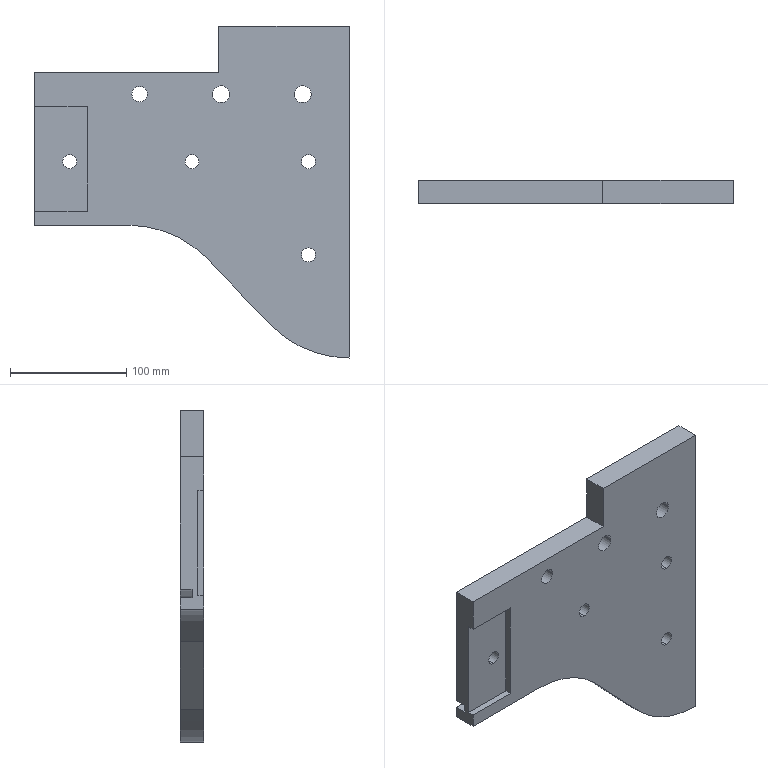Part | SolidWorks | features Cut 3, ICE 3, Extrusion 1 | 1 solid | 39 faces | box 270 x 20 x 285 mm | volume 953710 mm3 | cylinder 20 | plane 19 | commonest cylinder face diameters 12 x8 13.206 x2 14.603 x2 14.666 x2 190 x2 156 x1
STEP:
#1=CARTESIAN_POINT('',(-35.,0.,103.221));
#2=VERTEX_POINT('',#1);
#3=CARTESIAN_POINT('',(-35.,0.,91.221));
#4=VERTEX_POINT('',#3);
#5=CARTESIAN_POINT('',(-35.,0.,97.221));
#6=DIRECTION('',(0.,-1.,0.));
#7=DIRECTION('',(0.,0.,1.));
#8=AXIS2_PLACEMENT_3D('',#5,#6,#7);
#9=CIRCLE('',#8,6.);
#10=EDGE_CURVE('',#2,#4,#9,.T.);
#11=ORIENTED_EDGE('',*,*,#10,.T.);
#12=CARTESIAN_POINT('',(-35.,20.,91.221));
#13=VERTEX_POINT('',#12);
#14=CARTESIAN_POINT('',(-35.,-16.971,91.221));
#15=DIRECTION('',(0.,1.,0.));
#16=VECTOR('',#15,1000.);
#17=LINE('',#14,#16);
#18=EDGE_CURVE('',#4,#13,#17,.T.);
#19=ORIENTED_EDGE('',*,*,#18,.T.);
#20=CARTESIAN_POINT('',(-35.,20.,103.221));
#21=VERTEX_POINT('',#20);
#22=CARTESIAN_POINT('',(-35.,20.,97.221));
#23=DIRECTION('',(0.,1.,0.));
#24=DIRECTION('',(0.,0.,1.));
#25=AXIS2_PLACEMENT_3D('',#22,#23,#24);
#26=CIRCLE('',#25,6.);
#27=EDGE_CURVE('',#13,#21,#26,.T.);
#28=ORIENTED_EDGE('',*,*,#27,.T.);
#29=CARTESIAN_POINT('',(-35.,-16.971,103.221));
#30=DIRECTION('',(0.,1.,0.));
#31=VECTOR('',#30,1000.);
#32=LINE('',#29,#31);
#33=EDGE_CURVE('',#2,#21,#32,.T.);
#34=ORIENTED_EDGE('',*,*,#33,.F.);
#35=EDGE_LOOP('',(#11,#19,#28,#34));
#36=FACE_OUTER_BOUND('',#35,.T.);
#37=CARTESIAN_POINT('',(-35.,-16.971,97.221));
#38=DIRECTION('',(0.,1.,0.));
#39=DIRECTION('',(0.,0.,1.));
#40=AXIS2_PLACEMENT_3D('',#37,#38,#39);
#41=CYLINDRICAL_SURFACE('',#40,6.);
#42=ADVANCED_FACE('',(#36),#41,.F.);
#43=CARTESIAN_POINT('',(-32.667,0.,155.159));
#44=VERTEX_POINT('',#43);
#45=CARTESIAN_POINT('',(-47.333,0.,155.159));
#46=VERTEX_POINT('',#45);
#47=CARTESIAN_POINT('',(-40.,0.,155.159));
#48=DIRECTION('',(0.,1.,0.));
#49=DIRECTION('',(0.,0.,1.));
#50=AXIS2_PLACEMENT_3D('',#47,#48,#49);
#51=CIRCLE('',#50,7.333);
#52=EDGE_CURVE('',#44,#46,#51,.T.);
#53=ORIENTED_EDGE('',*,*,#52,.F.);
#54=CARTESIAN_POINT('',(-32.667,20.,155.159));
#55=VERTEX_POINT('',#54);
#56=CARTESIAN_POINT('',(-32.667,-30.741,155.159));
#57=DIRECTION('',(0.,1.,0.));
#58=VECTOR('',#57,1000.);
#59=LINE('',#56,#58);
#60=EDGE_CURVE('',#44,#55,#59,.T.);
#61=ORIENTED_EDGE('',*,*,#60,.T.);
#62=CARTESIAN_POINT('',(-47.333,20.,155.159));
#63=VERTEX_POINT('',#62);
#64=CARTESIAN_POINT('',(-40.,20.,155.159));
#65=DIRECTION('',(0.,1.,0.));
#66=DIRECTION('',(0.,0.,1.));
#67=AXIS2_PLACEMENT_3D('',#64,#65,#66);
#68=CIRCLE('',#67,7.333);
#69=EDGE_CURVE('',#55,#63,#68,.T.);
#70=ORIENTED_EDGE('',*,*,#69,.T.);
#71=CARTESIAN_POINT('',(-47.333,-30.741,155.159));
#72=DIRECTION('',(0.,1.,0.));
#73=VECTOR('',#72,1000.);
#74=LINE('',#71,#73);
#75=EDGE_CURVE('',#46,#63,#74,.T.);
#76=ORIENTED_EDGE('',*,*,#75,.F.);
#77=EDGE_LOOP('',(#53,#61,#70,#76));
#78=FACE_OUTER_BOUND('',#77,.T.);
#79=CARTESIAN_POINT('',(-40.,-30.741,155.159));
#80=DIRECTION('',(0.,1.,0.));
#81=DIRECTION('',(-1.,0.,0.));
#82=AXIS2_PLACEMENT_3D('',#79,#80,#81);
#83=CYLINDRICAL_SURFACE('',#82,7.333);
#84=ADVANCED_FACE('',(#78),#83,.F.);
#85=CARTESIAN_POINT('',(-102.699,0.,155.159));
#86=VERTEX_POINT('',#85);
#87=CARTESIAN_POINT('',(-117.301,0.,155.159));
#88=VERTEX_POINT('',#87);
#89=CARTESIAN_POINT('',(-110.,0.,155.159));
#90=DIRECTION('',(0.,1.,0.));
#91=DIRECTION('',(0.,0.,1.));
#92=AXIS2_PLACEMENT_3D('',#89,#90,#91);
#93=CIRCLE('',#92,7.301);
#94=EDGE_CURVE('',#86,#88,#93,.T.);
#95=ORIENTED_EDGE('',*,*,#94,.F.);
#96=CARTESIAN_POINT('',(-102.699,20.,155.159));
#97=VERTEX_POINT('',#96);
#98=CARTESIAN_POINT('',(-102.699,-30.741,155.159));
#99=DIRECTION('',(0.,1.,0.));
#100=VECTOR('',#99,1000.);
#101=LINE('',#98,#100);
#102=EDGE_CURVE('',#86,#97,#101,.T.);
#103=ORIENTED_EDGE('',*,*,#102,.T.);
#104=CARTESIAN_POINT('',(-117.301,20.,155.159));
#105=VERTEX_POINT('',#104);
#106=CARTESIAN_POINT('',(-110.,20.,155.159));
#107=DIRECTION('',(0.,1.,0.));
#108=DIRECTION('',(0.,0.,1.));
#109=AXIS2_PLACEMENT_3D('',#106,#107,#108);
#110=CIRCLE('',#109,7.301);
#111=EDGE_CURVE('',#97,#105,#110,.T.);
#112=ORIENTED_EDGE('',*,*,#111,.T.);
#113=CARTESIAN_POINT('',(-117.301,-30.741,155.159));
#114=DIRECTION('',(0.,1.,0.));
#115=VECTOR('',#114,1000.);
#116=LINE('',#113,#115);
#117=EDGE_CURVE('',#88,#105,#116,.T.);
#118=ORIENTED_EDGE('',*,*,#117,.F.);
#119=EDGE_LOOP('',(#95,#103,#112,#118));
#120=FACE_OUTER_BOUND('',#119,.T.);
#121=CARTESIAN_POINT('',(-110.,-30.741,155.159));
#122=DIRECTION('',(0.,1.,0.));
#123=DIRECTION('',(-1.,0.,0.));
#124=AXIS2_PLACEMENT_3D('',#121,#122,#123);
#125=CYLINDRICAL_SURFACE('',#124,7.301);
#126=ADVANCED_FACE('',(#120),#125,.F.);
#127=CARTESIAN_POINT('',(-173.397,0.,155.159));
#128=VERTEX_POINT('',#127);
#129=CARTESIAN_POINT('',(-186.603,0.,155.159));
#130=VERTEX_POINT('',#129);
#131=CARTESIAN_POINT('',(-180.,0.,155.159));
#132=DIRECTION('',(0.,1.,0.));
#133=DIRECTION('',(0.,0.,1.));
#134=AXIS2_PLACEMENT_3D('',#131,#132,#133);
#135=CIRCLE('',#134,6.603);
#136=EDGE_CURVE('',#128,#130,#135,.T.);
#137=ORIENTED_EDGE('',*,*,#136,.F.);
#138=CARTESIAN_POINT('',(-173.397,20.,155.159));
#139=VERTEX_POINT('',#138);
#140=CARTESIAN_POINT('',(-173.397,-30.741,155.159));
#141=DIRECTION('',(0.,1.,0.));
#142=VECTOR('',#141,1000.);
#143=LINE('',#140,#142);
#144=EDGE_CURVE('',#128,#139,#143,.T.);
#145=ORIENTED_EDGE('',*,*,#144,.T.);
#146=CARTESIAN_POINT('',(-186.603,20.,155.159));
#147=VERTEX_POINT('',#146);
#148=CARTESIAN_POINT('',(-180.,20.,155.159));
#149=DIRECTION('',(0.,1.,0.));
#150=DIRECTION('',(0.,0.,1.));
#151=AXIS2_PLACEMENT_3D('',#148,#149,#150);
#152=CIRCLE('',#151,6.603);
#153=EDGE_CURVE('',#139,#147,#152,.T.);
#154=ORIENTED_EDGE('',*,*,#153,.T.);
#155=CARTESIAN_POINT('',(-186.603,-30.741,155.159));
#156=DIRECTION('',(0.,1.,0.));
#157=VECTOR('',#156,1000.);
#158=LINE('',#155,#157);
#159=EDGE_CURVE('',#130,#147,#158,.T.);
#160=ORIENTED_EDGE('',*,*,#159,.F.);
#161=EDGE_LOOP('',(#137,#145,#154,#160));
#162=FACE_OUTER_BOUND('',#161,.T.);
#163=CARTESIAN_POINT('',(-180.,-30.741,155.159));
#164=DIRECTION('',(0.,1.,0.));
#165=DIRECTION('',(-1.,0.,0.));
#166=AXIS2_PLACEMENT_3D('',#163,#164,#165);
#167=CYLINDRICAL_SURFACE('',#166,6.603);
#168=ADVANCED_FACE('',(#162),#167,.F.);
#169=CARTESIAN_POINT('',(-35.,0.,23.221));
#170=VERTEX_POINT('',#169);
#171=CARTESIAN_POINT('',(-35.,0.,11.221));
#172=VERTEX_POINT('',#171);
#173=CARTESIAN_POINT('',(-35.,0.,17.221));
#174=DIRECTION('',(0.,-1.,0.));
#175=DIRECTION('',(0.,0.,1.));
#176=AXIS2_PLACEMENT_3D('',#173,#174,#175);
#177=CIRCLE('',#176,6.);
#178=EDGE_CURVE('',#170,#172,#177,.T.);
#179=ORIENTED_EDGE('',*,*,#178,.T.);
#180=CARTESIAN_POINT('',(-35.,20.,11.221));
#181=VERTEX_POINT('',#180);
#182=CARTESIAN_POINT('',(-35.,-16.971,11.221));
#183=DIRECTION('',(0.,1.,0.));
#184=VECTOR('',#183,1000.);
#185=LINE('',#182,#184);
#186=EDGE_CURVE('',#172,#181,#185,.T.);
#187=ORIENTED_EDGE('',*,*,#186,.T.);
#188=CARTESIAN_POINT('',(-35.,20.,23.221));
#189=VERTEX_POINT('',#188);
#190=CARTESIAN_POINT('',(-35.,20.,17.221));
#191=DIRECTION('',(0.,1.,0.));
#192=DIRECTION('',(0.,0.,1.));
#193=AXIS2_PLACEMENT_3D('',#190,#191,#192);
#194=CIRCLE('',#193,6.);
#195=EDGE_CURVE('',#181,#189,#194,.T.);
#196=ORIENTED_EDGE('',*,*,#195,.T.);
#197=CARTESIAN_POINT('',(-35.,-16.971,23.221));
#198=DIRECTION('',(0.,1.,0.));
#199=VECTOR('',#198,1000.);
#200=LINE('',#197,#199);
#201=EDGE_CURVE('',#170,#189,#200,.T.);
#202=ORIENTED_EDGE('',*,*,#201,.F.);
#203=EDGE_LOOP('',(#179,#187,#196,#202));
#204=FACE_OUTER_BOUND('',#203,.T.);
#205=CARTESIAN_POINT('',(-35.,-16.971,17.221));
#206=DIRECTION('',(0.,1.,0.));
#207=DIRECTION('',(0.,0.,1.));
#208=AXIS2_PLACEMENT_3D('',#205,#206,#207);
#209=CYLINDRICAL_SURFACE('',#208,6.);
#210=ADVANCED_FACE('',(#204),#209,.F.);
#211=CARTESIAN_POINT('',(-135.,0.,103.221));
#212=VERTEX_POINT('',#211);
#213=CARTESIAN_POINT('',(-135.,0.,91.221));
#214=VERTEX_POINT('',#213);
#215=CARTESIAN_POINT('',(-135.,0.,97.221));
#216=DIRECTION('',(0.,-1.,0.));
#217=DIRECTION('',(0.,0.,1.));
#218=AXIS2_PLACEMENT_3D('',#215,#216,#217);
#219=CIRCLE('',#218,6.);
#220=EDGE_CURVE('',#212,#214,#219,.T.);
#221=ORIENTED_EDGE('',*,*,#220,.T.);
#222=CARTESIAN_POINT('',(-135.,20.,91.221));
#223=VERTEX_POINT('',#222);
#224=CARTESIAN_POINT('',(-135.,-16.971,91.221));
#225=DIRECTION('',(0.,1.,0.));
#226=VECTOR('',#225,1000.);
#227=LINE('',#224,#226);
#228=EDGE_CURVE('',#214,#223,#227,.T.);
#229=ORIENTED_EDGE('',*,*,#228,.T.);
#230=CARTESIAN_POINT('',(-135.,20.,103.221));
#231=VERTEX_POINT('',#230);
#232=CARTESIAN_POINT('',(-135.,20.,97.221));
#233=DIRECTION('',(0.,1.,0.));
#234=DIRECTION('',(0.,0.,1.));
#235=AXIS2_PLACEMENT_3D('',#232,#233,#234);
#236=CIRCLE('',#235,6.);
#237=EDGE_CURVE('',#223,#231,#236,.T.);
#238=ORIENTED_EDGE('',*,*,#237,.T.);
#239=CARTESIAN_POINT('',(-135.,-16.971,103.221));
#240=DIRECTION('',(0.,1.,0.));
#241=VECTOR('',#240,1000.);
#242=LINE('',#239,#241);
#243=EDGE_CURVE('',#212,#231,#242,.T.);
#244=ORIENTED_EDGE('',*,*,#243,.F.);
#245=EDGE_LOOP('',(#221,#229,#238,#244));
#246=FACE_OUTER_BOUND('',#245,.T.);
#247=CARTESIAN_POINT('',(-135.,-16.971,97.221));
#248=DIRECTION('',(0.,1.,0.));
#249=DIRECTION('',(0.,0.,1.));
#250=AXIS2_PLACEMENT_3D('',#247,#248,#249);
#251=CYLINDRICAL_SURFACE('',#250,6.);
#252=ADVANCED_FACE('',(#246),#251,.F.);
#253=CARTESIAN_POINT('',(-240.,5.,103.221));
#254=VERTEX_POINT('',#253);
#255=CARTESIAN_POINT('',(-240.,5.,91.221));
#256=VERTEX_POINT('',#255);
#257=CARTESIAN_POINT('',(-240.,5.,97.221));
#258=DIRECTION('',(0.,-1.,0.));
#259=DIRECTION('',(0.,0.,-1.));
#260=AXIS2_PLACEMENT_3D('',#257,#258,#259);
#261=CIRCLE('',#260,6.);
#262=EDGE_CURVE('',#254,#256,#261,.T.);
#263=ORIENTED_EDGE('',*,*,#262,.T.);
#264=CARTESIAN_POINT('',(-240.,20.,91.221));
#265=VERTEX_POINT('',#264);
#266=CARTESIAN_POINT('',(-240.,-16.971,91.221));
#267=DIRECTION('',(0.,1.,0.));
#268=VECTOR('',#267,1000.);
#269=LINE('',#266,#268);
#270=EDGE_CURVE('',#256,#265,#269,.T.);
#271=ORIENTED_EDGE('',*,*,#270,.T.);
#272=CARTESIAN_POINT('',(-240.,20.,103.221));
#273=VERTEX_POINT('',#272);
#274=CARTESIAN_POINT('',(-240.,20.,97.221));
#275=DIRECTION('',(0.,1.,0.));
#276=DIRECTION('',(0.,0.,1.));
#277=AXIS2_PLACEMENT_3D('',#274,#275,#276);
#278=CIRCLE('',#277,6.);
#279=EDGE_CURVE('',#265,#273,#278,.T.);
#280=ORIENTED_EDGE('',*,*,#279,.T.);
#281=CARTESIAN_POINT('',(-240.,-16.971,103.221));
#282=DIRECTION('',(0.,1.,0.));
#283=VECTOR('',#282,1000.);
#284=LINE('',#281,#283);
#285=EDGE_CURVE('',#254,#273,#284,.T.);
#286=ORIENTED_EDGE('',*,*,#285,.F.);
#287=EDGE_LOOP('',(#263,#271,#280,#286));
#288=FACE_OUTER_BOUND('',#287,.T.);
#289=CARTESIAN_POINT('',(-240.,-16.971,97.221));
#290=DIRECTION('',(0.,1.,0.));
#291=DIRECTION('',(0.,0.,1.));
#292=AXIS2_PLACEMENT_3D('',#289,#290,#291);
#293=CYLINDRICAL_SURFACE('',#292,6.);
#294=ADVANCED_FACE('',(#288),#293,.F.);
#295=CARTESIAN_POINT('',(-112.,20.,173.659));
#296=VERTEX_POINT('',#295);
#297=CARTESIAN_POINT('',(-112.,0.,173.659));
#298=VERTEX_POINT('',#297);
#299=CARTESIAN_POINT('',(-112.,0.,173.659));
#300=DIRECTION('',(0.,-1.,0.));
#301=VECTOR('',#300,1000.);
#302=LINE('',#299,#301);
#303=EDGE_CURVE('',#296,#298,#302,.T.);
#304=ORIENTED_EDGE('',*,*,#303,.F.);
#305=CARTESIAN_POINT('',(-270.,20.,173.659));
#306=VERTEX_POINT('',#305);
#307=CARTESIAN_POINT('',(-270.,20.,173.659));
#308=DIRECTION('',(1.,0.,0.));
#309=VECTOR('',#308,1000.);
#310=LINE('',#307,#309);
#311=EDGE_CURVE('',#306,#296,#310,.T.);
#312=ORIENTED_EDGE('',*,*,#311,.F.);
#313=CARTESIAN_POINT('',(-270.,0.,173.659));
#314=VERTEX_POINT('',#313);
#315=CARTESIAN_POINT('',(-270.,20.,173.659));
#316=DIRECTION('',(0.,-1.,0.));
#317=VECTOR('',#316,1000.);
#318=LINE('',#315,#317);
#319=EDGE_CURVE('',#306,#314,#318,.T.);
#320=ORIENTED_EDGE('',*,*,#319,.T.);
#321=CARTESIAN_POINT('',(-190.,0.,173.659));
#322=DIRECTION('',(1.,0.,0.));
#323=VECTOR('',#322,1000.);
#324=LINE('',#321,#323);
#325=EDGE_CURVE('',#314,#298,#324,.T.);
#326=ORIENTED_EDGE('',*,*,#325,.T.);
#327=EDGE_LOOP('',(#304,#312,#320,#326));
#328=FACE_OUTER_BOUND('',#327,.T.);
#329=CARTESIAN_POINT('',(-190.,20.,173.659));
#330=DIRECTION('',(0.,0.,-1.));
#331=DIRECTION('',(-1.,0.,0.));
#332=AXIS2_PLACEMENT_3D('',#329,#330,#331);
#333=PLANE('',#332);
#334=ADVANCED_FACE('',(#328),#333,.F.);
#335=CARTESIAN_POINT('',(-190.,20.,52.659));
#336=VERTEX_POINT('',#335);
#337=CARTESIAN_POINT('',(-270.,20.,52.659));
#338=VERTEX_POINT('',#337);
#339=CARTESIAN_POINT('',(-270.,20.,52.659));
#340=DIRECTION('',(-1.,0.,0.));
#341=VECTOR('',#340,1000.);
#342=LINE('',#339,#341);
#343=EDGE_CURVE('',#336,#338,#342,.T.);
#344=ORIENTED_EDGE('',*,*,#343,.F.);
#345=CARTESIAN_POINT('',(-115.668,20.,21.82));
#346=VERTEX_POINT('',#345);
#347=CARTESIAN_POINT('',(-190.,20.,-52.341));
#348=DIRECTION('',(0.,-1.,0.));
#349=DIRECTION('',(0.,0.,1.));
#350=AXIS2_PLACEMENT_3D('',#347,#348,#349);
#351=CIRCLE('',#350,105.);
#352=EDGE_CURVE('',#346,#336,#351,.T.);
#353=ORIENTED_EDGE('',*,*,#352,.F.);
#354=CARTESIAN_POINT('',(-60.023,20.,-36.526));
#355=VERTEX_POINT('',#354);
#356=CARTESIAN_POINT('',(-115.668,20.,21.82));
#357=DIRECTION('',(-0.6902,0.,0.7237));
#358=VECTOR('',#357,1000.);
#359=LINE('',#356,#358);
#360=EDGE_CURVE('',#355,#346,#359,.T.);
#361=ORIENTED_EDGE('',*,*,#360,.F.);
#362=CARTESIAN_POINT('',(0.,20.,-61.341));
#363=VERTEX_POINT('',#362);
#364=CARTESIAN_POINT('',(0.,20.,23.659));
#365=DIRECTION('',(0.,1.,0.));
#366=DIRECTION('',(0.,0.,1.));
#367=AXIS2_PLACEMENT_3D('',#364,#365,#366);
#368=CIRCLE('',#367,85.);
#369=EDGE_CURVE('',#363,#355,#368,.T.);
#370=ORIENTED_EDGE('',*,*,#369,.F.);
#371=CARTESIAN_POINT('',(0.,20.,-71.341));
#372=VERTEX_POINT('',#371);
#373=CARTESIAN_POINT('',(0.,20.,173.659));
#374=DIRECTION('',(0.,0.,-1.));
#375=VECTOR('',#374,1000.);
#376=LINE('',#373,#375);
#377=EDGE_CURVE('',#363,#372,#376,.T.);
#378=ORIENTED_EDGE('',*,*,#377,.T.);
#379=CARTESIAN_POINT('',(-67.175,20.,-43.516));
#380=VERTEX_POINT('',#379);
#381=CARTESIAN_POINT('',(0.,20.,23.659));
#382=DIRECTION('',(0.,1.,0.));
#383=DIRECTION('',(0.,0.,1.));
#384=AXIS2_PLACEMENT_3D('',#381,#382,#383);
#385=CIRCLE('',#384,95.);
#386=EDGE_CURVE('',#372,#380,#385,.T.);
#387=ORIENTED_EDGE('',*,*,#386,.T.);
#388=CARTESIAN_POINT('',(-122.825,20.,14.835));
#389=VERTEX_POINT('',#388);
#390=CARTESIAN_POINT('',(-67.175,20.,-43.516));
#391=CARTESIAN_POINT('',(-95.,20.,-14.341));
#392=CARTESIAN_POINT('',(-122.825,20.,14.835));
#393=B_SPLINE_CURVE_WITH_KNOTS('',2,(#390,#391,#392),.UNSPECIFIED.,.F.,.F.,(3,3),(0.,1.),.UNSPECIFIED.);
#394=EDGE_CURVE('',#380,#389,#393,.T.);
#395=ORIENTED_EDGE('',*,*,#394,.T.);
#396=CARTESIAN_POINT('',(-190.,20.,42.659));
#397=VERTEX_POINT('',#396);
#398=CARTESIAN_POINT('',(-190.,20.,-52.341));
#399=DIRECTION('',(0.,-1.,0.));
#400=DIRECTION('',(0.,0.,1.));
#401=AXIS2_PLACEMENT_3D('',#398,#399,#400);
#402=CIRCLE('',#401,95.);
#403=EDGE_CURVE('',#389,#397,#402,.T.);
#404=ORIENTED_EDGE('',*,*,#403,.T.);
#405=CARTESIAN_POINT('',(-270.,20.,42.659));
#406=VERTEX_POINT('',#405);
#407=CARTESIAN_POINT('',(-270.,20.,42.659));
#408=DIRECTION('',(-1.,0.,0.));
#409=VECTOR('',#408,1000.);
#410=LINE('',#407,#409);
#411=EDGE_CURVE('',#397,#406,#410,.T.);
#412=ORIENTED_EDGE('',*,*,#411,.T.);
#413=CARTESIAN_POINT('',(-270.,20.,42.659));
#414=DIRECTION('',(0.,0.,1.));
#415=VECTOR('',#414,1000.);
#416=LINE('',#413,#415);
#417=EDGE_CURVE('',#406,#338,#416,.T.);
#418=ORIENTED_EDGE('',*,*,#417,.T.);
#419=EDGE_LOOP('',(#344,#353,#361,#370,#378,#387,#395,#404,#412,#418));
#420=FACE_OUTER_BOUND('',#419,.T.);
#421=CARTESIAN_POINT('',(-190.,20.,-52.341));
#422=DIRECTION('',(0.,1.,0.));
#423=DIRECTION('',(0.,0.,1.));
#424=AXIS2_PLACEMENT_3D('',#421,#422,#423);
#425=PLANE('',#424);
#426=ADVANCED_FACE('',(#420),#425,.T.);
#427=CARTESIAN_POINT('',(-122.825,0.,14.835));
#428=VERTEX_POINT('',#427);
#429=CARTESIAN_POINT('',(-190.,0.,42.659));
#430=VERTEX_POINT('',#429);
#431=CARTESIAN_POINT('',(-190.,0.,-52.341));
#432=DIRECTION('',(0.,-1.,0.));
#433=DIRECTION('',(0.,0.,1.));
#434=AXIS2_PLACEMENT_3D('',#431,#432,#433);
#435=CIRCLE('',#434,95.);
#436=EDGE_CURVE('',#428,#430,#435,.T.);
#437=ORIENTED_EDGE('',*,*,#436,.T.);
#438=CARTESIAN_POINT('',(-190.,20.,42.659));
#439=DIRECTION('',(0.,-1.,0.));
#440=VECTOR('',#439,1000.);
#441=LINE('',#438,#440);
#442=EDGE_CURVE('',#397,#430,#441,.T.);
#443=ORIENTED_EDGE('',*,*,#442,.F.);
#444=ORIENTED_EDGE('',*,*,#403,.F.);
#445=CARTESIAN_POINT('',(-122.825,20.,14.835));
#446=DIRECTION('',(0.,-1.,0.));
#447=VECTOR('',#446,1000.);
#448=LINE('',#445,#447);
#449=EDGE_CURVE('',#389,#428,#448,.T.);
#450=ORIENTED_EDGE('',*,*,#449,.T.);
#451=EDGE_LOOP('',(#437,#443,#444,#450));
#452=FACE_OUTER_BOUND('',#451,.T.);
#453=CARTESIAN_POINT('',(-190.,20.,-52.341));
#454=DIRECTION('',(0.,-1.,0.));
#455=DIRECTION('',(0.,0.,-1.));
#456=AXIS2_PLACEMENT_3D('',#453,#454,#455);
#457=CYLINDRICAL_SURFACE('',#456,95.);
#458=ADVANCED_FACE('',(#452),#457,.F.);
#459=CARTESIAN_POINT('',(-270.,0.,42.659));
#460=VERTEX_POINT('',#459);
#461=CARTESIAN_POINT('',(-270.,0.,42.659));
#462=DIRECTION('',(-1.,0.,0.));
#463=VECTOR('',#462,1000.);
#464=LINE('',#461,#463);
#465=EDGE_CURVE('',#430,#460,#464,.T.);
#466=ORIENTED_EDGE('',*,*,#465,.T.);
#467=CARTESIAN_POINT('',(-270.,20.,42.659));
#468=DIRECTION('',(0.,-1.,0.));
#469=VECTOR('',#468,1000.);
#470=LINE('',#467,#469);
#471=EDGE_CURVE('',#406,#460,#470,.T.);
#472=ORIENTED_EDGE('',*,*,#471,.F.);
#473=ORIENTED_EDGE('',*,*,#411,.F.);
#474=ORIENTED_EDGE('',*,*,#442,.T.);
#475=EDGE_LOOP('',(#466,#472,#473,#474));
#476=FACE_OUTER_BOUND('',#475,.T.);
#477=CARTESIAN_POINT('',(-270.,20.,42.659));
#478=DIRECTION('',(0.,0.,1.));
#479=DIRECTION('',(1.,0.,0.));
#480=AXIS2_PLACEMENT_3D('',#477,#478,#479);
#481=PLANE('',#480);
#482=ADVANCED_FACE('',(#476),#481,.F.);
#483=CARTESIAN_POINT('',(-270.,5.,144.659));
#484=VERTEX_POINT('',#483);
#485=CARTESIAN_POINT('',(-270.,5.,54.659));
#486=VERTEX_POINT('',#485);
#487=CARTESIAN_POINT('',(-270.,5.,144.659));
#488=DIRECTION('',(0.,0.,-1.));
#489=VECTOR('',#488,1000.);
#490=LINE('',#487,#489);
#491=EDGE_CURVE('',#484,#486,#490,.T.);
#492=ORIENTED_EDGE('',*,*,#491,.F.);
#493=CARTESIAN_POINT('',(-270.,0.,144.659));
#494=VERTEX_POINT('',#493);
#495=CARTESIAN_POINT('',(-270.,5.,144.659));
#496=DIRECTION('',(0.,-1.,0.));
#497=VECTOR('',#496,1000.);
#498=LINE('',#495,#497);
#499=EDGE_CURVE('',#484,#494,#498,.T.);
#500=ORIENTED_EDGE('',*,*,#499,.T.);
#501=CARTESIAN_POINT('',(-270.,0.,42.659));
#502=DIRECTION('',(0.,0.,1.));
#503=VECTOR('',#502,1000.);
#504=LINE('',#501,#503);
#505=EDGE_CURVE('',#494,#314,#504,.T.);
#506=ORIENTED_EDGE('',*,*,#505,.T.);
#507=ORIENTED_EDGE('',*,*,#319,.F.);
#508=CARTESIAN_POINT('',(-270.,20.,59.659));
#509=VERTEX_POINT('',#508);
#510=CARTESIAN_POINT('',(-270.,20.,42.659));
#511=DIRECTION('',(0.,0.,1.));
#512=VECTOR('',#511,1000.);
#513=LINE('',#510,#512);
#514=EDGE_CURVE('',#509,#306,#513,.T.);
#515=ORIENTED_EDGE('',*,*,#514,.F.);
#516=CARTESIAN_POINT('',(-270.,10.,59.659));
#517=VERTEX_POINT('',#516);
#518=CARTESIAN_POINT('',(-270.,10.,59.659));
#519=DIRECTION('',(0.,1.,0.));
#520=VECTOR('',#519,1000.);
#521=LINE('',#518,#520);
#522=EDGE_CURVE('',#517,#509,#521,.T.);
#523=ORIENTED_EDGE('',*,*,#522,.F.);
#524=CARTESIAN_POINT('',(-270.,10.,52.659));
#525=VERTEX_POINT('',#524);
#526=CARTESIAN_POINT('',(-270.,10.,52.659));
#527=DIRECTION('',(0.,0.,1.));
#528=VECTOR('',#527,1000.);
#529=LINE('',#526,#528);
#530=EDGE_CURVE('',#525,#517,#529,.T.);
#531=ORIENTED_EDGE('',*,*,#530,.F.);
#532=CARTESIAN_POINT('',(-270.,10.,52.659));
#533=DIRECTION('',(0.,1.,0.));
#534=VECTOR('',#533,1000.);
#535=LINE('',#532,#534);
#536=EDGE_CURVE('',#525,#338,#535,.T.);
#537=ORIENTED_EDGE('',*,*,#536,.T.);
#538=ORIENTED_EDGE('',*,*,#417,.F.);
#539=ORIENTED_EDGE('',*,*,#471,.T.);
#540=CARTESIAN_POINT('',(-270.,0.,54.659));
#541=VERTEX_POINT('',#540);
#542=CARTESIAN_POINT('',(-270.,0.,42.659));
#543=DIRECTION('',(0.,0.,1.));
#544=VECTOR('',#543,1000.);
#545=LINE('',#542,#544);
#546=EDGE_CURVE('',#460,#541,#545,.T.);
#547=ORIENTED_EDGE('',*,*,#546,.T.);
#548=CARTESIAN_POINT('',(-270.,5.,54.659));
#549=DIRECTION('',(0.,-1.,0.));
#550=VECTOR('',#549,1000.);
#551=LINE('',#548,#550);
#552=EDGE_CURVE('',#486,#541,#551,.T.);
#553=ORIENTED_EDGE('',*,*,#552,.F.);
#554=EDGE_LOOP('',(#492,#500,#506,#507,#515,#523,#531,#537,#538,#539,#547,#553));
#555=FACE_OUTER_BOUND('',#554,.T.);
#556=CARTESIAN_POINT('',(-270.,20.,42.659));
#557=DIRECTION('',(1.,0.,0.));
#558=DIRECTION('',(0.,0.,-1.));
#559=AXIS2_PLACEMENT_3D('',#556,#557,#558);
#560=PLANE('',#559);
#561=ADVANCED_FACE('',(#555),#560,.F.);
#562=ORIENTED_EDGE('',*,*,#377,.F.);
#563=CARTESIAN_POINT('',(0.,10.,-61.341));
#564=VERTEX_POINT('',#563);
#565=CARTESIAN_POINT('',(0.,10.,-61.341));
#566=DIRECTION('',(0.,1.,0.));
#567=VECTOR('',#566,1000.);
#568=LINE('',#565,#567);
#569=EDGE_CURVE('',#564,#363,#568,.T.);
#570=ORIENTED_EDGE('',*,*,#569,.F.);
#571=CARTESIAN_POINT('',(0.,10.,-54.341));
#572=VERTEX_POINT('',#571);
#573=CARTESIAN_POINT('',(0.,10.,-61.341));
#574=DIRECTION('',(0.,0.,-1.));
#575=VECTOR('',#574,1000.);
#576=LINE('',#573,#575);
#577=EDGE_CURVE('',#572,#564,#576,.T.);
#578=ORIENTED_EDGE('',*,*,#577,.F.);
#579=CARTESIAN_POINT('',(0.,20.,-54.341));
#580=VERTEX_POINT('',#579);
#581=CARTESIAN_POINT('',(0.,10.,-54.341));
#582=DIRECTION('',(0.,1.,0.));
#583=VECTOR('',#582,1000.);
#584=LINE('',#581,#583);
#585=EDGE_CURVE('',#572,#580,#584,.T.);
#586=ORIENTED_EDGE('',*,*,#585,.T.);
#587=CARTESIAN_POINT('',(0.,20.,213.659));
#588=VERTEX_POINT('',#587);
#589=CARTESIAN_POINT('',(0.,20.,173.659));
#590=DIRECTION('',(0.,0.,-1.));
#591=VECTOR('',#590,1000.);
#592=LINE('',#589,#591);
#593=EDGE_CURVE('',#588,#580,#592,.T.);
#594=ORIENTED_EDGE('',*,*,#593,.F.);
#595=CARTESIAN_POINT('',(0.,0.,213.659));
#596=VERTEX_POINT('',#595);
#597=CARTESIAN_POINT('',(0.,0.,213.659));
#598=DIRECTION('',(0.,1.,0.));
#599=VECTOR('',#598,1000.);
#600=LINE('',#597,#599);
#601=EDGE_CURVE('',#596,#588,#600,.T.);
#602=ORIENTED_EDGE('',*,*,#601,.F.);
#603=CARTESIAN_POINT('',(0.,0.,-71.341));
#604=VERTEX_POINT('',#603);
#605=CARTESIAN_POINT('',(0.,0.,173.659));
#606=DIRECTION('',(0.,0.,-1.));
#607=VECTOR('',#606,1000.);
#608=LINE('',#605,#607);
#609=EDGE_CURVE('',#596,#604,#608,.T.);
#610=ORIENTED_EDGE('',*,*,#609,.T.);
#611=CARTESIAN_POINT('',(0.,20.,-71.341));
#612=DIRECTION('',(0.,-1.,0.));
#613=VECTOR('',#612,1000.);
#614=LINE('',#611,#613);
#615=EDGE_CURVE('',#372,#604,#614,.T.);
#616=ORIENTED_EDGE('',*,*,#615,.F.);
#617=EDGE_LOOP('',(#562,#570,#578,#586,#594,#602,#610,#616));
#618=FACE_OUTER_BOUND('',#617,.T.);
#619=CARTESIAN_POINT('',(0.,20.,173.659));
#620=DIRECTION('',(-1.,0.,0.));
#621=DIRECTION('',(0.,0.,1.));
#622=AXIS2_PLACEMENT_3D('',#619,#620,#621);
#623=PLANE('',#622);
#624=ADVANCED_FACE('',(#618),#623,.F.);
#625=CARTESIAN_POINT('',(-67.175,0.,-43.516));
#626=VERTEX_POINT('',#625);
#627=CARTESIAN_POINT('',(0.,0.,23.659));
#628=DIRECTION('',(0.,1.,0.));
#629=DIRECTION('',(0.,0.,1.));
#630=AXIS2_PLACEMENT_3D('',#627,#628,#629);
#631=CIRCLE('',#630,95.);
#632=EDGE_CURVE('',#604,#626,#631,.T.);
#633=ORIENTED_EDGE('',*,*,#632,.T.);
#634=CARTESIAN_POINT('',(-67.175,20.,-43.516));
#635=DIRECTION('',(0.,-1.,0.));
#636=VECTOR('',#635,1000.);
#637=LINE('',#634,#636);
#638=EDGE_CURVE('',#380,#626,#637,.T.);
#639=ORIENTED_EDGE('',*,*,#638,.F.);
#640=ORIENTED_EDGE('',*,*,#386,.F.);
#641=ORIENTED_EDGE('',*,*,#615,.T.);
#642=EDGE_LOOP('',(#633,#639,#640,#641));
#643=FACE_OUTER_BOUND('',#642,.T.);
#644=CARTESIAN_POINT('',(0.,20.,23.659));
#645=DIRECTION('',(0.,-1.,0.));
#646=DIRECTION('',(0.,0.,-1.));
#647=AXIS2_PLACEMENT_3D('',#644,#645,#646);
#648=CYLINDRICAL_SURFACE('',#647,95.);
#649=ADVANCED_FACE('',(#643),#648,.T.);
#650=CARTESIAN_POINT('',(-67.175,0.,-43.516));
#651=CARTESIAN_POINT('',(-95.,0.,-14.341));
#652=CARTESIAN_POINT('',(-122.825,0.,14.835));
#653=B_SPLINE_CURVE_WITH_KNOTS('',2,(#650,#651,#652),.UNSPECIFIED.,.F.,.F.,(3,3),(0.,1.),.UNSPECIFIED.);
#654=EDGE_CURVE('',#626,#428,#653,.T.);
#655=ORIENTED_EDGE('',*,*,#654,.T.);
#656=ORIENTED_EDGE('',*,*,#449,.F.);
#657=ORIENTED_EDGE('',*,*,#394,.F.);
#658=ORIENTED_EDGE('',*,*,#638,.T.);
#659=EDGE_LOOP('',(#655,#656,#657,#658));
#660=FACE_OUTER_BOUND('',#659,.T.);
#661=CARTESIAN_POINT('',(-67.175,20.,-43.516));
#662=DIRECTION('',(0.7237,0.,0.6902));
#663=DIRECTION('',(0.6902,0.,-0.7237));
#664=AXIS2_PLACEMENT_3D('',#661,#662,#663);
#665=PLANE('',#664);
#666=ADVANCED_FACE('',(#660),#665,.F.);
#667=CARTESIAN_POINT('',(-35.,20.,97.221));
#668=DIRECTION('',(0.,1.,0.));
#669=DIRECTION('',(0.,0.,1.));
#670=AXIS2_PLACEMENT_3D('',#667,#668,#669);
#671=CIRCLE('',#670,6.);
#672=EDGE_CURVE('',#21,#13,#671,.T.);
#673=ORIENTED_EDGE('',*,*,#672,.F.);
#674=ORIENTED_EDGE('',*,*,#27,.F.);
#675=EDGE_LOOP('',(#673,#674));
#676=FACE_BOUND('',#675,.T.);
#677=CARTESIAN_POINT('',(-40.,20.,155.159));
#678=DIRECTION('',(0.,1.,0.));
#679=DIRECTION('',(0.,0.,1.));
#680=AXIS2_PLACEMENT_3D('',#677,#678,#679);
#681=CIRCLE('',#680,7.333);
#682=EDGE_CURVE('',#63,#55,#681,.T.);
#683=ORIENTED_EDGE('',*,*,#682,.F.);
#684=ORIENTED_EDGE('',*,*,#69,.F.);
#685=EDGE_LOOP('',(#683,#684));
#686=FACE_BOUND('',#685,.T.);
#687=CARTESIAN_POINT('',(-110.,20.,155.159));
#688=DIRECTION('',(0.,1.,0.));
#689=DIRECTION('',(0.,0.,1.));
#690=AXIS2_PLACEMENT_3D('',#687,#688,#689);
#691=CIRCLE('',#690,7.301);
#692=EDGE_CURVE('',#105,#97,#691,.T.);
#693=ORIENTED_EDGE('',*,*,#692,.F.);
#694=ORIENTED_EDGE('',*,*,#111,.F.);
#695=EDGE_LOOP('',(#693,#694));
#696=FACE_BOUND('',#695,.T.);
#697=CARTESIAN_POINT('',(-180.,20.,155.159));
#698=DIRECTION('',(0.,1.,0.));
#699=DIRECTION('',(0.,0.,1.));
#700=AXIS2_PLACEMENT_3D('',#697,#698,#699);
#701=CIRCLE('',#700,6.603);
#702=EDGE_CURVE('',#147,#139,#701,.T.);
#703=ORIENTED_EDGE('',*,*,#702,.F.);
#704=ORIENTED_EDGE('',*,*,#153,.F.);
#705=EDGE_LOOP('',(#703,#704));
#706=FACE_BOUND('',#705,.T.);
#707=CARTESIAN_POINT('',(-35.,20.,17.221));
#708=DIRECTION('',(0.,1.,0.));
#709=DIRECTION('',(0.,0.,1.));
#710=AXIS2_PLACEMENT_3D('',#707,#708,#709);
#711=CIRCLE('',#710,6.);
#712=EDGE_CURVE('',#189,#181,#711,.T.);
#713=ORIENTED_EDGE('',*,*,#712,.F.);
#714=ORIENTED_EDGE('',*,*,#195,.F.);
#715=EDGE_LOOP('',(#713,#714));
#716=FACE_BOUND('',#715,.T.);
#717=CARTESIAN_POINT('',(-240.,20.,97.221));
#718=DIRECTION('',(0.,1.,0.));
#719=DIRECTION('',(0.,0.,1.));
#720=AXIS2_PLACEMENT_3D('',#717,#718,#719);
#721=CIRCLE('',#720,6.);
#722=EDGE_CURVE('',#273,#265,#721,.T.);
#723=ORIENTED_EDGE('',*,*,#722,.F.);
#724=ORIENTED_EDGE('',*,*,#279,.F.);
#725=EDGE_LOOP('',(#723,#724));
#726=FACE_BOUND('',#725,.T.);
#727=CARTESIAN_POINT('',(-135.,20.,97.221));
#728=DIRECTION('',(0.,1.,0.));
#729=DIRECTION('',(0.,0.,1.));
#730=AXIS2_PLACEMENT_3D('',#727,#728,#729);
#731=CIRCLE('',#730,6.);
#732=EDGE_CURVE('',#231,#223,#731,.T.);
#733=ORIENTED_EDGE('',*,*,#732,.F.);
#734=ORIENTED_EDGE('',*,*,#237,.F.);
#735=EDGE_LOOP('',(#733,#734));
#736=FACE_BOUND('',#735,.T.);
#737=CARTESIAN_POINT('',(-55.019,20.,-31.63));
#738=VERTEX_POINT('',#737);
#739=CARTESIAN_POINT('',(0.,20.,23.659));
#740=DIRECTION('',(0.,-1.,0.));
#741=DIRECTION('',(0.,0.,1.));
#742=AXIS2_PLACEMENT_3D('',#739,#740,#741);
#743=CIRCLE('',#742,78.);
#744=EDGE_CURVE('',#738,#580,#743,.T.);
#745=ORIENTED_EDGE('',*,*,#744,.F.);
#746=CARTESIAN_POINT('',(-110.656,20.,26.707));
#747=VERTEX_POINT('',#746);
#748=CARTESIAN_POINT('',(-110.656,20.,26.707));
#749=DIRECTION('',(0.6902,0.,-0.7237));
#750=VECTOR('',#749,1000.);
#751=LINE('',#748,#750);
#752=EDGE_CURVE('',#747,#738,#751,.T.);
#753=ORIENTED_EDGE('',*,*,#752,.F.);
#754=CARTESIAN_POINT('',(-190.,20.,59.659));
#755=VERTEX_POINT('',#754);
#756=CARTESIAN_POINT('',(-190.,20.,-52.341));
#757=DIRECTION('',(0.,1.,0.));
#758=DIRECTION('',(0.,0.,1.));
#759=AXIS2_PLACEMENT_3D('',#756,#757,#758);
#760=CIRCLE('',#759,112.);
#761=EDGE_CURVE('',#755,#747,#760,.T.);
#762=ORIENTED_EDGE('',*,*,#761,.F.);
#763=CARTESIAN_POINT('',(-270.,20.,59.659));
#764=DIRECTION('',(1.,0.,0.));
#765=VECTOR('',#764,1000.);
#766=LINE('',#763,#765);
#767=EDGE_CURVE('',#509,#755,#766,.T.);
#768=ORIENTED_EDGE('',*,*,#767,.F.);
#769=ORIENTED_EDGE('',*,*,#514,.T.);
#770=ORIENTED_EDGE('',*,*,#311,.T.);
#771=CARTESIAN_POINT('',(-112.,20.,213.659));
#772=VERTEX_POINT('',#771);
#773=CARTESIAN_POINT('',(-112.,20.,213.659));
#774=DIRECTION('',(0.,0.,-1.));
#775=VECTOR('',#774,1000.);
#776=LINE('',#773,#775);
#777=EDGE_CURVE('',#772,#296,#776,.T.);
#778=ORIENTED_EDGE('',*,*,#777,.F.);
#779=CARTESIAN_POINT('',(0.,20.,213.659));
#780=DIRECTION('',(-1.,0.,0.));
#781=VECTOR('',#780,1000.);
#782=LINE('',#779,#781);
#783=EDGE_CURVE('',#588,#772,#782,.T.);
#784=ORIENTED_EDGE('',*,*,#783,.F.);
#785=ORIENTED_EDGE('',*,*,#593,.T.);
#786=EDGE_LOOP('',(#745,#753,#762,#768,#769,#770,#778,#784,#785));
#787=FACE_OUTER_BOUND('',#786,.T.);
#788=CARTESIAN_POINT('',(-190.,20.,-52.341));
#789=DIRECTION('',(0.,1.,0.));
#790=DIRECTION('',(0.,0.,1.));
#791=AXIS2_PLACEMENT_3D('',#788,#789,#790);
#792=PLANE('',#791);
#793=ADVANCED_FACE('',(#676,#686,#696,#706,#716,#726,#736,#787),#792,.T.);
#794=ORIENTED_EDGE('',*,*,#10,.F.);
#795=CARTESIAN_POINT('',(-35.,0.,97.221));
#796=DIRECTION('',(0.,-1.,0.));
#797=DIRECTION('',(0.,0.,1.));
#798=AXIS2_PLACEMENT_3D('',#795,#796,#797);
#799=CIRCLE('',#798,6.);
#800=EDGE_CURVE('',#4,#2,#799,.T.);
#801=ORIENTED_EDGE('',*,*,#800,.F.);
#802=EDGE_LOOP('',(#794,#801));
#803=FACE_BOUND('',#802,.T.);
#804=CARTESIAN_POINT('',(-40.,0.,155.159));
#805=DIRECTION('',(0.,1.,0.));
#806=DIRECTION('',(0.,0.,1.));
#807=AXIS2_PLACEMENT_3D('',#804,#805,#806);
#808=CIRCLE('',#807,7.333);
#809=EDGE_CURVE('',#46,#44,#808,.T.);
#810=ORIENTED_EDGE('',*,*,#809,.T.);
#811=ORIENTED_EDGE('',*,*,#52,.T.);
#812=EDGE_LOOP('',(#810,#811));
#813=FACE_BOUND('',#812,.T.);
#814=CARTESIAN_POINT('',(-110.,0.,155.159));
#815=DIRECTION('',(0.,1.,0.));
#816=DIRECTION('',(0.,0.,1.));
#817=AXIS2_PLACEMENT_3D('',#814,#815,#816);
#818=CIRCLE('',#817,7.301);
#819=EDGE_CURVE('',#88,#86,#818,.T.);
#820=ORIENTED_EDGE('',*,*,#819,.T.);
#821=ORIENTED_EDGE('',*,*,#94,.T.);
#822=EDGE_LOOP('',(#820,#821));
#823=FACE_BOUND('',#822,.T.);
#824=CARTESIAN_POINT('',(-180.,0.,155.159));
#825=DIRECTION('',(0.,1.,0.));
#826=DIRECTION('',(0.,0.,1.));
#827=AXIS2_PLACEMENT_3D('',#824,#825,#826);
#828=CIRCLE('',#827,6.603);
#829=EDGE_CURVE('',#130,#128,#828,.T.);
#830=ORIENTED_EDGE('',*,*,#829,.T.);
#831=ORIENTED_EDGE('',*,*,#136,.T.);
#832=EDGE_LOOP('',(#830,#831));
#833=FACE_BOUND('',#832,.T.);
#834=ORIENTED_EDGE('',*,*,#178,.F.);
#835=CARTESIAN_POINT('',(-35.,0.,17.221));
#836=DIRECTION('',(0.,-1.,0.));
#837=DIRECTION('',(0.,0.,1.));
#838=AXIS2_PLACEMENT_3D('',#835,#836,#837);
#839=CIRCLE('',#838,6.);
#840=EDGE_CURVE('',#172,#170,#839,.T.);
#841=ORIENTED_EDGE('',*,*,#840,.F.);
#842=EDGE_LOOP('',(#834,#841));
#843=FACE_BOUND('',#842,.T.);
#844=ORIENTED_EDGE('',*,*,#220,.F.);
#845=CARTESIAN_POINT('',(-135.,0.,97.221));
#846=DIRECTION('',(0.,-1.,0.));
#847=DIRECTION('',(0.,0.,1.));
#848=AXIS2_PLACEMENT_3D('',#845,#846,#847);
#849=CIRCLE('',#848,6.);
#850=EDGE_CURVE('',#214,#212,#849,.T.);
#851=ORIENTED_EDGE('',*,*,#850,.F.);
#852=EDGE_LOOP('',(#844,#851));
#853=FACE_BOUND('',#852,.T.);
#854=ORIENTED_EDGE('',*,*,#505,.F.);
#855=CARTESIAN_POINT('',(-225.,0.,144.659));
#856=VERTEX_POINT('',#855);
#857=CARTESIAN_POINT('',(-225.,0.,144.659));
#858=DIRECTION('',(-1.,0.,0.));
#859=VECTOR('',#858,1000.);
#860=LINE('',#857,#859);
#861=EDGE_CURVE('',#856,#494,#860,.T.);
#862=ORIENTED_EDGE('',*,*,#861,.F.);
#863=CARTESIAN_POINT('',(-225.,0.,54.659));
#864=VERTEX_POINT('',#863);
#865=CARTESIAN_POINT('',(-225.,0.,54.659));
#866=DIRECTION('',(0.,0.,1.));
#867=VECTOR('',#866,1000.);
#868=LINE('',#865,#867);
#869=EDGE_CURVE('',#864,#856,#868,.T.);
#870=ORIENTED_EDGE('',*,*,#869,.F.);
#871=CARTESIAN_POINT('',(-270.,0.,54.659));
#872=DIRECTION('',(1.,0.,0.));
#873=VECTOR('',#872,1000.);
#874=LINE('',#871,#873);
#875=EDGE_CURVE('',#541,#864,#874,.T.);
#876=ORIENTED_EDGE('',*,*,#875,.F.);
#877=ORIENTED_EDGE('',*,*,#546,.F.);
#878=ORIENTED_EDGE('',*,*,#465,.F.);
#879=ORIENTED_EDGE('',*,*,#436,.F.);
#880=ORIENTED_EDGE('',*,*,#654,.F.);
#881=ORIENTED_EDGE('',*,*,#632,.F.);
#882=ORIENTED_EDGE('',*,*,#609,.F.);
#883=CARTESIAN_POINT('',(-112.,0.,213.659));
#884=VERTEX_POINT('',#883);
#885=CARTESIAN_POINT('',(0.,0.,213.659));
#886=DIRECTION('',(1.,0.,0.));
#887=VECTOR('',#886,1000.);
#888=LINE('',#885,#887);
#889=EDGE_CURVE('',#884,#596,#888,.T.);
#890=ORIENTED_EDGE('',*,*,#889,.F.);
#891=CARTESIAN_POINT('',(-112.,0.,213.659));
#892=DIRECTION('',(0.,0.,-1.));
#893=VECTOR('',#892,1000.);
#894=LINE('',#891,#893);
#895=EDGE_CURVE('',#884,#298,#894,.T.);
#896=ORIENTED_EDGE('',*,*,#895,.T.);
#897=ORIENTED_EDGE('',*,*,#325,.F.);
#898=EDGE_LOOP('',(#854,#862,#870,#876,#877,#878,#879,#880,#881,#882,#890,#896,#897));
#899=FACE_OUTER_BOUND('',#898,.T.);
#900=CARTESIAN_POINT('',(-190.,0.,-52.341));
#901=DIRECTION('',(0.,1.,0.));
#902=DIRECTION('',(0.,0.,1.));
#903=AXIS2_PLACEMENT_3D('',#900,#901,#902);
#904=PLANE('',#903);
#905=ADVANCED_FACE('',(#803,#813,#823,#833,#843,#853,#899),#904,.F.);
#906=ORIENTED_EDGE('',*,*,#343,.T.);
#907=ORIENTED_EDGE('',*,*,#536,.F.);
#908=CARTESIAN_POINT('',(-190.,10.,52.659));
#909=VERTEX_POINT('',#908);
#910=CARTESIAN_POINT('',(-270.,10.,52.659));
#911=DIRECTION('',(-1.,0.,0.));
#912=VECTOR('',#911,1000.);
#913=LINE('',#910,#912);
#914=EDGE_CURVE('',#909,#525,#913,.T.);
#915=ORIENTED_EDGE('',*,*,#914,.F.);
#916=CARTESIAN_POINT('',(-190.,10.,52.659));
#917=DIRECTION('',(0.,1.,0.));
#918=VECTOR('',#917,1000.);
#919=LINE('',#916,#918);
#920=EDGE_CURVE('',#909,#336,#919,.T.);
#921=ORIENTED_EDGE('',*,*,#920,.T.);
#922=EDGE_LOOP('',(#906,#907,#915,#921));
#923=FACE_OUTER_BOUND('',#922,.T.);
#924=CARTESIAN_POINT('',(-270.,10.,52.659));
#925=DIRECTION('',(0.,0.,-1.));
#926=DIRECTION('',(-1.,0.,0.));
#927=AXIS2_PLACEMENT_3D('',#924,#925,#926);
#928=PLANE('',#927);
#929=ADVANCED_FACE('',(#923),#928,.F.);
#930=ORIENTED_EDGE('',*,*,#352,.T.);
#931=ORIENTED_EDGE('',*,*,#920,.F.);
#932=CARTESIAN_POINT('',(-115.668,10.,21.82));
#933=VERTEX_POINT('',#932);
#934=CARTESIAN_POINT('',(-190.,10.,-52.341));
#935=DIRECTION('',(0.,-1.,0.));
#936=DIRECTION('',(0.,0.,1.));
#937=AXIS2_PLACEMENT_3D('',#934,#935,#936);
#938=CIRCLE('',#937,105.);
#939=EDGE_CURVE('',#933,#909,#938,.T.);
#940=ORIENTED_EDGE('',*,*,#939,.F.);
#941=CARTESIAN_POINT('',(-115.668,10.,21.82));
#942=DIRECTION('',(0.,1.,0.));
#943=VECTOR('',#942,1000.);
#944=LINE('',#941,#943);
#945=EDGE_CURVE('',#933,#346,#944,.T.);
#946=ORIENTED_EDGE('',*,*,#945,.T.);
#947=EDGE_LOOP('',(#930,#931,#940,#946));
#948=FACE_OUTER_BOUND('',#947,.T.);
#949=CARTESIAN_POINT('',(-190.,10.,-52.341));
#950=DIRECTION('',(0.,1.,0.));
#951=DIRECTION('',(0.,0.,1.));
#952=AXIS2_PLACEMENT_3D('',#949,#950,#951);
#953=CYLINDRICAL_SURFACE('',#952,105.);
#954=ADVANCED_FACE('',(#948),#953,.T.);
#955=ORIENTED_EDGE('',*,*,#360,.T.);
#956=ORIENTED_EDGE('',*,*,#945,.F.);
#957=CARTESIAN_POINT('',(-60.023,10.,-36.526));
#958=VERTEX_POINT('',#957);
#959=CARTESIAN_POINT('',(-115.668,10.,21.82));
#960=DIRECTION('',(-0.6902,0.,0.7237));
#961=VECTOR('',#960,1000.);
#962=LINE('',#959,#961);
#963=EDGE_CURVE('',#958,#933,#962,.T.);
#964=ORIENTED_EDGE('',*,*,#963,.F.);
#965=CARTESIAN_POINT('',(-60.023,10.,-36.526));
#966=DIRECTION('',(0.,1.,0.));
#967=VECTOR('',#966,1000.);
#968=LINE('',#965,#967);
#969=EDGE_CURVE('',#958,#355,#968,.T.);
#970=ORIENTED_EDGE('',*,*,#969,.T.);
#971=EDGE_LOOP('',(#955,#956,#964,#970));
#972=FACE_OUTER_BOUND('',#971,.T.);
#973=CARTESIAN_POINT('',(-115.668,10.,21.82));
#974=DIRECTION('',(-0.7237,0.,-0.6902));
#975=DIRECTION('',(-0.6902,0.,0.7237));
#976=AXIS2_PLACEMENT_3D('',#973,#974,#975);
#977=PLANE('',#976);
#978=ADVANCED_FACE('',(#972),#977,.F.);
#979=ORIENTED_EDGE('',*,*,#369,.T.);
#980=ORIENTED_EDGE('',*,*,#969,.F.);
#981=CARTESIAN_POINT('',(0.,10.,23.659));
#982=DIRECTION('',(0.,1.,0.));
#983=DIRECTION('',(0.,0.,1.));
#984=AXIS2_PLACEMENT_3D('',#981,#982,#983);
#985=CIRCLE('',#984,85.);
#986=EDGE_CURVE('',#564,#958,#985,.T.);
#987=ORIENTED_EDGE('',*,*,#986,.F.);
#988=ORIENTED_EDGE('',*,*,#569,.T.);
#989=EDGE_LOOP('',(#979,#980,#987,#988));
#990=FACE_OUTER_BOUND('',#989,.T.);
#991=CARTESIAN_POINT('',(0.,10.,23.659));
#992=DIRECTION('',(0.,1.,0.));
#993=DIRECTION('',(0.,0.,1.));
#994=AXIS2_PLACEMENT_3D('',#991,#992,#993);
#995=CYLINDRICAL_SURFACE('',#994,85.);
#996=ADVANCED_FACE('',(#990),#995,.F.);
#997=ORIENTED_EDGE('',*,*,#744,.T.);
#998=ORIENTED_EDGE('',*,*,#585,.F.);
#999=CARTESIAN_POINT('',(-55.019,10.,-31.63));
#1000=VERTEX_POINT('',#999);
#1001=CARTESIAN_POINT('',(0.,10.,23.659));
#1002=DIRECTION('',(0.,-1.,0.));
#1003=DIRECTION('',(0.,0.,1.));
#1004=AXIS2_PLACEMENT_3D('',#1001,#1002,#1003);
#1005=CIRCLE('',#1004,78.);
#1006=EDGE_CURVE('',#1000,#572,#1005,.T.);
#1007=ORIENTED_EDGE('',*,*,#1006,.F.);
#1008=CARTESIAN_POINT('',(-55.019,10.,-31.63));
#1009=DIRECTION('',(0.,1.,0.));
#1010=VECTOR('',#1009,1000.);
#1011=LINE('',#1008,#1010);
#1012=EDGE_CURVE('',#1000,#738,#1011,.T.);
#1013=ORIENTED_EDGE('',*,*,#1012,.T.);
#1014=EDGE_LOOP('',(#997,#998,#1007,#1013));
#1015=FACE_OUTER_BOUND('',#1014,.T.);
#1016=CARTESIAN_POINT('',(0.,10.,23.659));
#1017=DIRECTION('',(0.,1.,0.));
#1018=DIRECTION('',(0.,0.,1.));
#1019=AXIS2_PLACEMENT_3D('',#1016,#1017,#1018);
#1020=CYLINDRICAL_SURFACE('',#1019,78.);
#1021=ADVANCED_FACE('',(#1015),#1020,.T.);
#1022=ORIENTED_EDGE('',*,*,#752,.T.);
#1023=ORIENTED_EDGE('',*,*,#1012,.F.);
#1024=CARTESIAN_POINT('',(-110.656,10.,26.707));
#1025=VERTEX_POINT('',#1024);
#1026=CARTESIAN_POINT('',(-110.656,10.,26.707));
#1027=DIRECTION('',(0.6902,0.,-0.7237));
#1028=VECTOR('',#1027,1000.);
#1029=LINE('',#1026,#1028);
#1030=EDGE_CURVE('',#1025,#1000,#1029,.T.);
#1031=ORIENTED_EDGE('',*,*,#1030,.F.);
#1032=CARTESIAN_POINT('',(-110.656,10.,26.707));
#1033=DIRECTION('',(0.,1.,0.));
#1034=VECTOR('',#1033,1000.);
#1035=LINE('',#1032,#1034);
#1036=EDGE_CURVE('',#1025,#747,#1035,.T.);
#1037=ORIENTED_EDGE('',*,*,#1036,.T.);
#1038=EDGE_LOOP('',(#1022,#1023,#1031,#1037));
#1039=FACE_OUTER_BOUND('',#1038,.T.);
#1040=CARTESIAN_POINT('',(-110.656,10.,26.707));
#1041=DIRECTION('',(0.7237,0.,0.6902));
#1042=DIRECTION('',(0.6902,0.,-0.7237));
#1043=AXIS2_PLACEMENT_3D('',#1040,#1041,#1042);
#1044=PLANE('',#1043);
#1045=ADVANCED_FACE('',(#1039),#1044,.F.);
#1046=ORIENTED_EDGE('',*,*,#761,.T.);
#1047=ORIENTED_EDGE('',*,*,#1036,.F.);
#1048=CARTESIAN_POINT('',(-190.,10.,59.659));
#1049=VERTEX_POINT('',#1048);
#1050=CARTESIAN_POINT('',(-190.,10.,-52.341));
#1051=DIRECTION('',(0.,1.,0.));
#1052=DIRECTION('',(0.,0.,1.));
#1053=AXIS2_PLACEMENT_3D('',#1050,#1051,#1052);
#1054=CIRCLE('',#1053,112.);
#1055=EDGE_CURVE('',#1049,#1025,#1054,.T.);
#1056=ORIENTED_EDGE('',*,*,#1055,.F.);
#1057=CARTESIAN_POINT('',(-190.,10.,59.659));
#1058=DIRECTION('',(0.,1.,0.));
#1059=VECTOR('',#1058,1000.);
#1060=LINE('',#1057,#1059);
#1061=EDGE_CURVE('',#1049,#755,#1060,.T.);
#1062=ORIENTED_EDGE('',*,*,#1061,.T.);
#1063=EDGE_LOOP('',(#1046,#1047,#1056,#1062));
#1064=FACE_OUTER_BOUND('',#1063,.T.);
#1065=CARTESIAN_POINT('',(-190.,10.,-52.341));
#1066=DIRECTION('',(0.,1.,0.));
#1067=DIRECTION('',(0.,0.,1.));
#1068=AXIS2_PLACEMENT_3D('',#1065,#1066,#1067);
#1069=CYLINDRICAL_SURFACE('',#1068,112.);
#1070=ADVANCED_FACE('',(#1064),#1069,.F.);
#1071=ORIENTED_EDGE('',*,*,#767,.T.);
#1072=ORIENTED_EDGE('',*,*,#1061,.F.);
#1073=CARTESIAN_POINT('',(-270.,10.,59.659));
#1074=DIRECTION('',(1.,0.,0.));
#1075=VECTOR('',#1074,1000.);
#1076=LINE('',#1073,#1075);
#1077=EDGE_CURVE('',#517,#1049,#1076,.T.);
#1078=ORIENTED_EDGE('',*,*,#1077,.F.);
#1079=ORIENTED_EDGE('',*,*,#522,.T.);
#1080=EDGE_LOOP('',(#1071,#1072,#1078,#1079));
#1081=FACE_OUTER_BOUND('',#1080,.T.);
#1082=CARTESIAN_POINT('',(-270.,10.,59.659));
#1083=DIRECTION('',(0.,0.,1.));
#1084=DIRECTION('',(1.,0.,0.));
#1085=AXIS2_PLACEMENT_3D('',#1082,#1083,#1084);
#1086=PLANE('',#1085);
#1087=ADVANCED_FACE('',(#1081),#1086,.F.);
#1088=ORIENTED_EDGE('',*,*,#530,.T.);
#1089=ORIENTED_EDGE('',*,*,#1077,.T.);
#1090=ORIENTED_EDGE('',*,*,#1055,.T.);
#1091=ORIENTED_EDGE('',*,*,#1030,.T.);
#1092=ORIENTED_EDGE('',*,*,#1006,.T.);
#1093=ORIENTED_EDGE('',*,*,#577,.T.);
#1094=ORIENTED_EDGE('',*,*,#986,.T.);
#1095=ORIENTED_EDGE('',*,*,#963,.T.);
#1096=ORIENTED_EDGE('',*,*,#939,.T.);
#1097=ORIENTED_EDGE('',*,*,#914,.T.);
#1098=EDGE_LOOP('',(#1088,#1089,#1090,#1091,#1092,#1093,#1094,#1095,#1096,#1097));
#1099=FACE_OUTER_BOUND('',#1098,.T.);
#1100=CARTESIAN_POINT('',(-190.,10.,-52.341));
#1101=DIRECTION('',(0.,1.,0.));
#1102=DIRECTION('',(0.,0.,1.));
#1103=AXIS2_PLACEMENT_3D('',#1100,#1101,#1102);
#1104=PLANE('',#1103);
#1105=ADVANCED_FACE('',(#1099),#1104,.T.);
#1106=ORIENTED_EDGE('',*,*,#861,.T.);
#1107=ORIENTED_EDGE('',*,*,#499,.F.);
#1108=CARTESIAN_POINT('',(-225.,5.,144.659));
#1109=VERTEX_POINT('',#1108);
#1110=CARTESIAN_POINT('',(-225.,5.,144.659));
#1111=DIRECTION('',(-1.,0.,0.));
#1112=VECTOR('',#1111,1000.);
#1113=LINE('',#1110,#1112);
#1114=EDGE_CURVE('',#1109,#484,#1113,.T.);
#1115=ORIENTED_EDGE('',*,*,#1114,.F.);
#1116=CARTESIAN_POINT('',(-225.,5.,144.659));
#1117=DIRECTION('',(0.,-1.,0.));
#1118=VECTOR('',#1117,1000.);
#1119=LINE('',#1116,#1118);
#1120=EDGE_CURVE('',#1109,#856,#1119,.T.);
#1121=ORIENTED_EDGE('',*,*,#1120,.T.);
#1122=EDGE_LOOP('',(#1106,#1107,#1115,#1121));
#1123=FACE_OUTER_BOUND('',#1122,.T.);
#1124=CARTESIAN_POINT('',(-225.,5.,144.659));
#1125=DIRECTION('',(0.,0.,1.));
#1126=DIRECTION('',(1.,0.,0.));
#1127=AXIS2_PLACEMENT_3D('',#1124,#1125,#1126);
#1128=PLANE('',#1127);
#1129=ADVANCED_FACE('',(#1123),#1128,.F.);
#1130=ORIENTED_EDGE('',*,*,#869,.T.);
#1131=ORIENTED_EDGE('',*,*,#1120,.F.);
#1132=CARTESIAN_POINT('',(-225.,5.,54.659));
#1133=VERTEX_POINT('',#1132);
#1134=CARTESIAN_POINT('',(-225.,5.,54.659));
#1135=DIRECTION('',(0.,0.,1.));
#1136=VECTOR('',#1135,1000.);
#1137=LINE('',#1134,#1136);
#1138=EDGE_CURVE('',#1133,#1109,#1137,.T.);
#1139=ORIENTED_EDGE('',*,*,#1138,.F.);
#1140=CARTESIAN_POINT('',(-225.,5.,54.659));
#1141=DIRECTION('',(0.,-1.,0.));
#1142=VECTOR('',#1141,1000.);
#1143=LINE('',#1140,#1142);
#1144=EDGE_CURVE('',#1133,#864,#1143,.T.);
#1145=ORIENTED_EDGE('',*,*,#1144,.T.);
#1146=EDGE_LOOP('',(#1130,#1131,#1139,#1145));
#1147=FACE_OUTER_BOUND('',#1146,.T.);
#1148=CARTESIAN_POINT('',(-225.,5.,54.659));
#1149=DIRECTION('',(1.,0.,0.));
#1150=DIRECTION('',(0.,0.,-1.));
#1151=AXIS2_PLACEMENT_3D('',#1148,#1149,#1150);
#1152=PLANE('',#1151);
#1153=ADVANCED_FACE('',(#1147),#1152,.F.);
#1154=ORIENTED_EDGE('',*,*,#875,.T.);
#1155=ORIENTED_EDGE('',*,*,#1144,.F.);
#1156=CARTESIAN_POINT('',(-270.,5.,54.659));
#1157=DIRECTION('',(1.,0.,0.));
#1158=VECTOR('',#1157,1000.);
#1159=LINE('',#1156,#1158);
#1160=EDGE_CURVE('',#486,#1133,#1159,.T.);
#1161=ORIENTED_EDGE('',*,*,#1160,.F.);
#1162=ORIENTED_EDGE('',*,*,#552,.T.);
#1163=EDGE_LOOP('',(#1154,#1155,#1161,#1162));
#1164=FACE_OUTER_BOUND('',#1163,.T.);
#1165=CARTESIAN_POINT('',(-270.,5.,54.659));
#1166=DIRECTION('',(0.,0.,-1.));
#1167=DIRECTION('',(-1.,0.,0.));
#1168=AXIS2_PLACEMENT_3D('',#1165,#1166,#1167);
#1169=PLANE('',#1168);
#1170=ADVANCED_FACE('',(#1164),#1169,.F.);
#1171=ORIENTED_EDGE('',*,*,#262,.F.);
#1172=CARTESIAN_POINT('',(-240.,5.,97.221));
#1173=DIRECTION('',(0.,-1.,0.));
#1174=DIRECTION('',(0.,0.,-1.));
#1175=AXIS2_PLACEMENT_3D('',#1172,#1173,#1174);
#1176=CIRCLE('',#1175,6.);
#1177=EDGE_CURVE('',#256,#254,#1176,.T.);
#1178=ORIENTED_EDGE('',*,*,#1177,.F.);
#1179=EDGE_LOOP('',(#1171,#1178));
#1180=FACE_BOUND('',#1179,.T.);
#1181=ORIENTED_EDGE('',*,*,#491,.T.);
#1182=ORIENTED_EDGE('',*,*,#1160,.T.);
#1183=ORIENTED_EDGE('',*,*,#1138,.T.);
#1184=ORIENTED_EDGE('',*,*,#1114,.T.);
#1185=EDGE_LOOP('',(#1181,#1182,#1183,#1184));
#1186=FACE_OUTER_BOUND('',#1185,.T.);
#1187=CARTESIAN_POINT('',(0.,5.,0.));
#1188=DIRECTION('',(0.,-1.,0.));
#1189=DIRECTION('',(0.,0.,-1.));
#1190=AXIS2_PLACEMENT_3D('',#1187,#1188,#1189);
#1191=PLANE('',#1190);
#1192=ADVANCED_FACE('',(#1180,#1186),#1191,.T.);
#1193=ORIENTED_EDGE('',*,*,#303,.T.);
#1194=ORIENTED_EDGE('',*,*,#895,.F.);
#1195=CARTESIAN_POINT('',(-112.,0.,213.659));
#1196=DIRECTION('',(0.,-1.,0.));
#1197=VECTOR('',#1196,1000.);
#1198=LINE('',#1195,#1197);
#1199=EDGE_CURVE('',#772,#884,#1198,.T.);
#1200=ORIENTED_EDGE('',*,*,#1199,.F.);
#1201=ORIENTED_EDGE('',*,*,#777,.T.);
#1202=EDGE_LOOP('',(#1193,#1194,#1200,#1201));
#1203=FACE_OUTER_BOUND('',#1202,.T.);
#1204=CARTESIAN_POINT('',(-112.,0.,213.659));
#1205=DIRECTION('',(1.,0.,0.));
#1206=DIRECTION('',(0.,0.,-1.));
#1207=AXIS2_PLACEMENT_3D('',#1204,#1205,#1206);
#1208=PLANE('',#1207);
#1209=ADVANCED_FACE('',(#1203),#1208,.F.);
#1210=ORIENTED_EDGE('',*,*,#601,.T.);
#1211=ORIENTED_EDGE('',*,*,#783,.T.);
#1212=ORIENTED_EDGE('',*,*,#1199,.T.);
#1213=ORIENTED_EDGE('',*,*,#889,.T.);
#1214=EDGE_LOOP('',(#1210,#1211,#1212,#1213));
#1215=FACE_OUTER_BOUND('',#1214,.T.);
#1216=CARTESIAN_POINT('',(0.,0.,213.659));
#1217=DIRECTION('',(0.,0.,1.));
#1218=DIRECTION('',(1.,0.,0.));
#1219=AXIS2_PLACEMENT_3D('',#1216,#1217,#1218);
#1220=PLANE('',#1219);
#1221=ADVANCED_FACE('',(#1215),#1220,.T.);
#1222=ORIENTED_EDGE('',*,*,#270,.F.);
#1223=ORIENTED_EDGE('',*,*,#1177,.T.);
#1224=ORIENTED_EDGE('',*,*,#285,.T.);
#1225=ORIENTED_EDGE('',*,*,#722,.T.);
#1226=EDGE_LOOP('',(#1222,#1223,#1224,#1225));
#1227=FACE_OUTER_BOUND('',#1226,.T.);
#1228=CARTESIAN_POINT('',(-240.,-16.971,97.221));
#1229=DIRECTION('',(0.,1.,0.));
#1230=DIRECTION('',(0.,0.,1.));
#1231=AXIS2_PLACEMENT_3D('',#1228,#1229,#1230);
#1232=CYLINDRICAL_SURFACE('',#1231,6.);
#1233=ADVANCED_FACE('',(#1227),#1232,.F.);
#1234=ORIENTED_EDGE('',*,*,#228,.F.);
#1235=ORIENTED_EDGE('',*,*,#850,.T.);
#1236=ORIENTED_EDGE('',*,*,#243,.T.);
#1237=ORIENTED_EDGE('',*,*,#732,.T.);
#1238=EDGE_LOOP('',(#1234,#1235,#1236,#1237));
#1239=FACE_OUTER_BOUND('',#1238,.T.);
#1240=CARTESIAN_POINT('',(-135.,-16.971,97.221));
#1241=DIRECTION('',(0.,1.,0.));
#1242=DIRECTION('',(0.,0.,1.));
#1243=AXIS2_PLACEMENT_3D('',#1240,#1241,#1242);
#1244=CYLINDRICAL_SURFACE('',#1243,6.);
#1245=ADVANCED_FACE('',(#1239),#1244,.F.);
#1246=ORIENTED_EDGE('',*,*,#186,.F.);
#1247=ORIENTED_EDGE('',*,*,#840,.T.);
#1248=ORIENTED_EDGE('',*,*,#201,.T.);
#1249=ORIENTED_EDGE('',*,*,#712,.T.);
#1250=EDGE_LOOP('',(#1246,#1247,#1248,#1249));
#1251=FACE_OUTER_BOUND('',#1250,.T.);
#1252=CARTESIAN_POINT('',(-35.,-16.971,17.221));
#1253=DIRECTION('',(0.,1.,0.));
#1254=DIRECTION('',(0.,0.,1.));
#1255=AXIS2_PLACEMENT_3D('',#1252,#1253,#1254);
#1256=CYLINDRICAL_SURFACE('',#1255,6.);
#1257=ADVANCED_FACE('',(#1251),#1256,.F.);
#1258=ORIENTED_EDGE('',*,*,#144,.F.);
#1259=ORIENTED_EDGE('',*,*,#829,.F.);
#1260=ORIENTED_EDGE('',*,*,#159,.T.);
#1261=ORIENTED_EDGE('',*,*,#702,.T.);
#1262=EDGE_LOOP('',(#1258,#1259,#1260,#1261));
#1263=FACE_OUTER_BOUND('',#1262,.T.);
#1264=CARTESIAN_POINT('',(-180.,-30.741,155.159));
#1265=DIRECTION('',(0.,1.,0.));
#1266=DIRECTION('',(-1.,0.,0.));
#1267=AXIS2_PLACEMENT_3D('',#1264,#1265,#1266);
#1268=CYLINDRICAL_SURFACE('',#1267,6.603);
#1269=ADVANCED_FACE('',(#1263),#1268,.F.);
#1270=ORIENTED_EDGE('',*,*,#102,.F.);
#1271=ORIENTED_EDGE('',*,*,#819,.F.);
#1272=ORIENTED_EDGE('',*,*,#117,.T.);
#1273=ORIENTED_EDGE('',*,*,#692,.T.);
#1274=EDGE_LOOP('',(#1270,#1271,#1272,#1273));
#1275=FACE_OUTER_BOUND('',#1274,.T.);
#1276=CARTESIAN_POINT('',(-110.,-30.741,155.159));
#1277=DIRECTION('',(0.,1.,0.));
#1278=DIRECTION('',(-1.,0.,0.));
#1279=AXIS2_PLACEMENT_3D('',#1276,#1277,#1278);
#1280=CYLINDRICAL_SURFACE('',#1279,7.301);
#1281=ADVANCED_FACE('',(#1275),#1280,.F.);
#1282=ORIENTED_EDGE('',*,*,#60,.F.);
#1283=ORIENTED_EDGE('',*,*,#809,.F.);
#1284=ORIENTED_EDGE('',*,*,#75,.T.);
#1285=ORIENTED_EDGE('',*,*,#682,.T.);
#1286=EDGE_LOOP('',(#1282,#1283,#1284,#1285));
#1287=FACE_OUTER_BOUND('',#1286,.T.);
#1288=CARTESIAN_POINT('',(-40.,-30.741,155.159));
#1289=DIRECTION('',(0.,1.,0.));
#1290=DIRECTION('',(-1.,0.,0.));
#1291=AXIS2_PLACEMENT_3D('',#1288,#1289,#1290);
#1292=CYLINDRICAL_SURFACE('',#1291,7.333);
#1293=ADVANCED_FACE('',(#1287),#1292,.F.);
#1294=ORIENTED_EDGE('',*,*,#18,.F.);
#1295=ORIENTED_EDGE('',*,*,#800,.T.);
#1296=ORIENTED_EDGE('',*,*,#33,.T.);
#1297=ORIENTED_EDGE('',*,*,#672,.T.);
#1298=EDGE_LOOP('',(#1294,#1295,#1296,#1297));
#1299=FACE_OUTER_BOUND('',#1298,.T.);
#1300=CARTESIAN_POINT('',(-35.,-16.971,97.221));
#1301=DIRECTION('',(0.,1.,0.));
#1302=DIRECTION('',(0.,0.,1.));
#1303=AXIS2_PLACEMENT_3D('',#1300,#1301,#1302);
#1304=CYLINDRICAL_SURFACE('',#1303,6.);
#1305=ADVANCED_FACE('',(#1299),#1304,.F.);
#1306=CLOSED_SHELL('',(#42,#84,#126,#168,#210,#252,#294,#334,#426,#458,#482,#561,#624,#649,#666,#793,#905,#929,#954,#978,#996,#1021,#1045,#1070,#1087,#1105,#1129,#1153,#1170,#1192,#1209,#1221,#1233,#1245,#1257,#1269,#1281,#1293,#1305));
#1307=MANIFOLD_SOLID_BREP('',#1306);
#1308=CARTESIAN_POINT('',(0.,0.,0.));
#1309=DIRECTION('',(0.,0.,1.));
#1310=DIRECTION('',(1.,0.,0.));
#1311=AXIS2_PLACEMENT_3D('',#1308,#1309,#1310);
#1312=(LENGTH_UNIT()NAMED_UNIT(*)SI_UNIT(.MILLI.,.METRE.));
#1313=UNCERTAINTY_MEASURE_WITH_UNIT(LENGTH_MEASURE(0.00001),#1312,'','');
#1314=(NAMED_UNIT(*)PLANE_ANGLE_UNIT()SI_UNIT($,.RADIAN.));
#1315=(NAMED_UNIT(*)SI_UNIT($,.STERADIAN.)SOLID_ANGLE_UNIT());
#1316=(GEOMETRIC_REPRESENTATION_CONTEXT(3)GLOBAL_UNCERTAINTY_ASSIGNED_CONTEXT((#1313))GLOBAL_UNIT_ASSIGNED_CONTEXT((#1312,#1314,#1315))REPRESENTATION_CONTEXT('',''));
#1317=ADVANCED_BREP_SHAPE_REPRESENTATION('',(#1307,#1311),#1316);